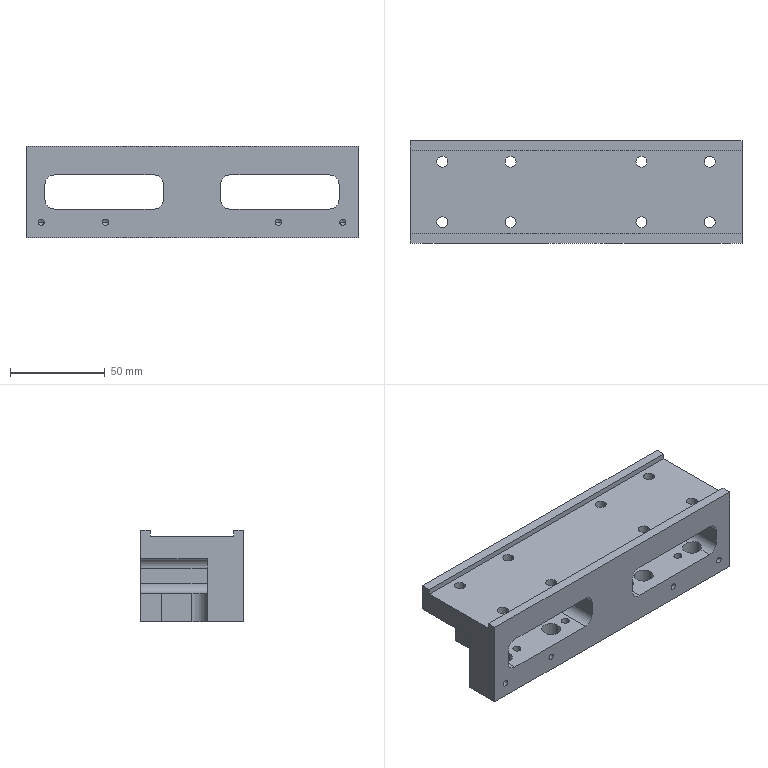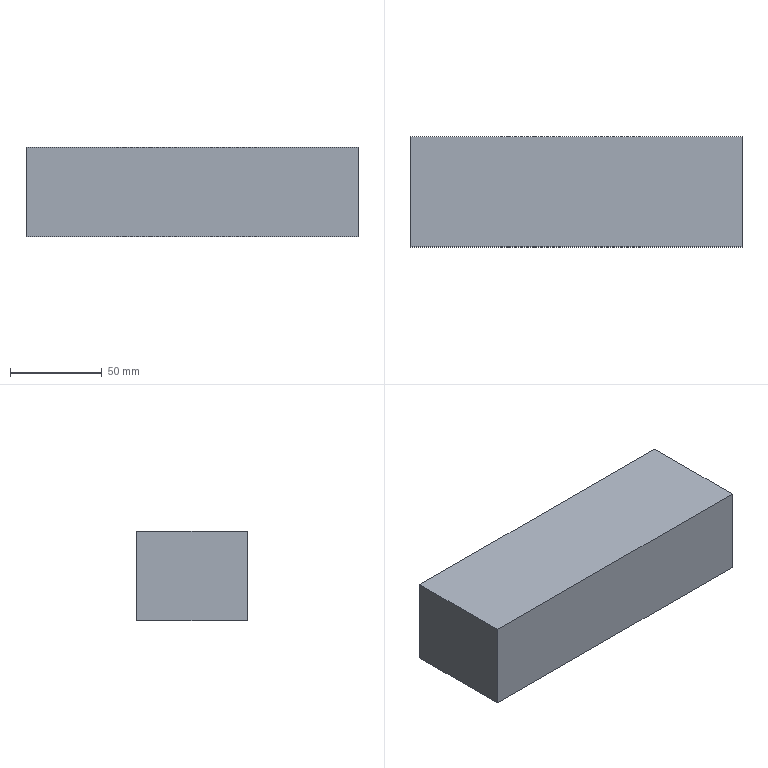CAM job | NX | 3+2 milling, drilling | part box 175 x 54 x 48 mm | stock box 181 x 60 x 49 mm
Tools:
number,name,description,diameter,corner_radius,flute_length,length,flutes
1,D50,Milling Tool-5 Parameters,50.0,0.0,50.0,75.0,2
3,D10,Milling Tool-5 Parameters,10.0,0.0,50.0,75.0,2
2,D6A45,Milling Tool-5 Parameters,6.0,0.0,3.0,3.0,2
15,5.8ZT,Drilling Tool,5.8,0.0,35.0,50.0,2
4,D10JING,Milling Tool-5 Parameters,10.0,0.0,50.0,75.0,2
13,3.3ZT,Drilling Tool,3.3,0.0,35.0,50.0,2
17,M4,Milling Tool-5 Parameters,3.3,0.0,30.0,30.0,4
Operations:
program,operation,operation_type,tool,method,geometry_group,spindle_rpm,surface_speed,feed_per_tooth,feed_cut,feed_plunge,cut_length_mm,path_length_mm,cut_time_min,machine_time_min
1-178-55-50毛胚,FLOOR_WALL,VolumeBased25DMillingOperation,D50,METHOD,A,6500.0,1286.0,0.0962,1250.0,100.0,513.997,533.997,0.4112,0.4132
1-178-55-50毛胚,ADAPTIVE_MILLING,CavityMilling,D10,METHOD,A,7000.0,219.0,0.1571,2200.0,1000.0,25455.236,27474.037,11.587,11.789
1-178-55-50毛胚,DRILLING_COPY_1,Operation,D6A45,METHOD,A,3000.0,56.0,0.0333,200.0,0.0,40.8,438.476,0.204,0.2438
1-178-55-50毛胚,DRILLING_COPY_1_COPY_COPY_COPY_COPY,Operation,5.8ZT,METHOD,A,2000.0,20.0,0.0375,150.0,0.0,125.94,608.756,0.8396,0.8879
1-178-55-50毛胚,FLOOR_WALL_1_COPY_1,VolumeBased25DMillingOperation,D10JING,METHOD,A,7000.0,87.0,0.0714,1000.0,100.0,1906.84,1969.344,1.907,1.915
1-178-55-50毛胚,ZLEVEL_PROFILE_COPY_COPY_1_COPY_COPY_COPY_1,ZLevelMilling,D10JING,METHOD,A,7000.0,219.0,0.0714,1000.0,100.0,1477.645,1595.961,1.478,1.49
1-178-55-50毛胚,ZLEVEL_PROFILE_COPY_1_COPY_COPY_COPY_COPY_2_COPY,ZLevelMilling,D6A45,METHOD,A,7000.0,131.0,0.0714,1000.0,1000.0,738.212,970.506,0.7382,0.7614
1-178-55-50毛胚,ZLEVEL_PROFILE_COPY_1_COPY_COPY_COPY_COPY_2_COPY_COPY,ZLevelMilling,D6A45,METHOD,A,7000.0,131.0,0.0714,1000.0,1000.0,204.794,1242.78,0.2048,0.3086
1-178-55-50毛胚,刀补4,VolumeBased25DMillingOperation,D10JING,METHOD,A,7000.0,87.0,0.0714,1000.0,100.0,385.208,444.12,0.3852,0.3931
2-178-55-50毛胚,DRILLING_COPY_1_COPY,Operation,D6A45,METHOD,B,3000.0,56.0,0.0333,200.0,0.0,20.4,269.114,0.102,0.1269
2-178-55-50毛胚,DRILLING_COPY_1_COPY_COPY_COPY_COPY_COPY,Operation,3.3ZT,METHOD,B,2000.0,20.0,0.0375,150.0,0.0,56.366,409.024,0.3758,0.411
2-178-55-50毛胚,DRILLING_COPY_1_COPY_COPY_COPY_COPY_COPY_COPY,Operation,M4,METHOD,B,200.0,2.0,0.175,140.0,0.0,52.4,333.114,0.3743,0.4024
2-178-55-50毛胚,ZLEVEL_PROFILE,ZLevelMilling,D10,METHOD,B,7000.0,219.0,0.1429,2000.0,1000.0,13195.642,13494.934,6.646,6.676
2-178-55-50毛胚,ZLEVEL_PROFILE_COPY_COPY_1_COPY_COPY_COPY_1_COPY,ZLevelMilling,D10JING,METHOD,B,7000.0,219.0,0.0714,1000.0,100.0,745.498,1224.468,0.7455,0.7934
2-178-55-50毛胚,ZLEVEL_PROFILE_COPY_1_COPY_COPY_COPY_COPY_2_COPY_COPY_COPY,ZLevelMilling,D6A45,METHOD,B,7000.0,131.0,0.0714,1000.0,1000.0,779.045,1870.996,0.779,0.8882